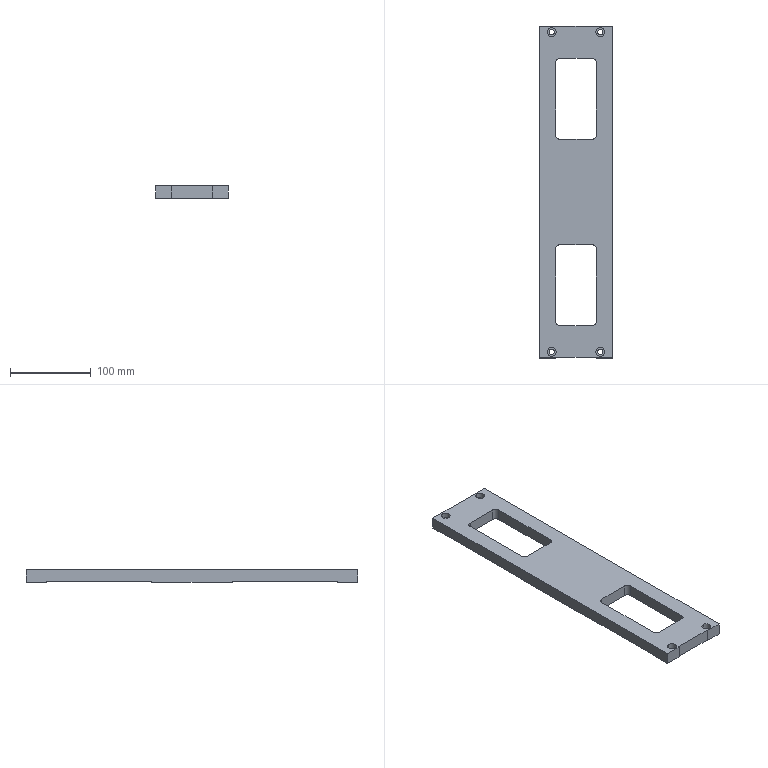NC program | NX | posted with a generic post | part box 90 x 410 x 15 mm
Whole program:
N10 G17 G21 G94 G90
(PLANAR_MILL_1_COPY_COPY , TOOL : D6A45)
N12 T07 M6
N14 G54
N16 G17 G0 G90 X-200.57 Y-28.539 S9500 M3
N18 G43 Z30. H7
N20 Z0.5
N22 G94 G1 Z-1. F1250.
N24 X-201.6 Y-29.134
N26 G3 X-202.1 Y-30. R1.
N28 X-197.5 Y-34.6 R4.6
N30 X-202.1 Y-30. R-4.6
N32 X-201.6 Y-30.866 R1.
N34 G1 X-200.57 Y-31.461
N36 Z0.5
N38 G0 Z30.
N40 Y31.461
N42 Z0.5
N44 G1 Z-1.
N46 X-201.6 Y30.866
N48 G3 X-202.1 Y30. R1.
N50 X-197.5 Y25.4 R4.6
N52 X-202.1 Y30. R-4.6
N54 X-201.6 Y29.134 R1.
N56 G1 X-200.57 Y28.539
N58 Z0.5
N60 G0 Z30.
N62 X-113.73 Y22.9
N64 Z0.5
N66 G1 Z-1.
N68 X-114.134 Y23.6
N70 G3 X-115. Y24.1 R1.
N72 G1 X-160.
N74 G3 X-164.1 Y20. R4.1
N76 G1 Y-20.
N78 G3 X-160. Y-24.1 R4.1
N80 G1 X-70.
N82 G3 X-65.9 Y-20. R4.1
N84 G1 Y20.
N86 G3 X-70. Y24.1 R4.1
N88 G1 X-115.
N90 G3 X-115.866 Y23.6 R1.
N92 G1 X-116.27 Y22.9
N94 Z0.5
N96 G0 Z30.
N98 X-1.27 Y47.1
N100 Z0.5
N102 G1 Z-1.
N104 X-0.866 Y46.4
N106 G3 X0. Y45.9 R1.
N108 G1 X204.9
N110 G2 X205.9 Y44.9 R1.
N112 G1 Y25.1
N114 G2 X204.9 Y24.1 R1.
N116 G1 Y-24.1
N118 G2 X205.9 Y-25.1 R1.
N120 G1 Y-44.9
N122 G2 X204.9 Y-45.9 R1.
N124 G1 X-204.9
N126 G2 X-205.9 Y-44.9 R1.
N128 G1 Y44.9
N130 G2 X-204.9 Y45.9 R1.
N132 G1 X0.
N134 G3 X0.866 Y46.4 R1.
N136 G1 X1.27 Y47.1
N138 Z0.5
N140 G0 Z30.
N142 X116.27 Y22.9
N144 Z0.5
N146 G1 Z-1.
N148 X115.866 Y23.6
N150 G3 X115. Y24.1 R1.
N152 G1 X70.
N154 G3 X65.9 Y20. R4.1
N156 G1 Y-20.
N158 G3 X70. Y-24.1 R4.1
N160 G1 X160.
N162 G3 X164.1 Y-20. R4.1
N164 G1 Y20.
N166 G3 X160. Y24.1 R4.1
N168 G1 X115.
N170 G3 X114.134 Y23.6 R1.
N172 G1 X113.73 Y22.9
N174 Z0.5
N176 G0 Z30.
N178 X200.57 Y28.539
N180 Z0.5
N182 G1 Z-1.
N184 X201.6 Y29.134
N186 G3 X202.1 Y30. R1.
N188 X197.5 Y34.6 R4.6
N190 X202.1 Y30. R-4.6
N192 X201.6 Y30.866 R1.
N194 G1 X200.57 Y31.461
N196 Z0.5
N198 G0 Z30.
N200 Y-31.461
N202 Z0.5
N204 G1 Z-1.
N206 X201.6 Y-30.866
N208 G3 X202.1 Y-30. R1.
N210 X197.5 Y-25.4 R4.6
N212 X202.1 Y-30. R-4.6
N214 X201.6 Y-29.134 R1.
N216 G1 X200.57 Y-28.539
N218 Z0.5
N220 G0 Z30.
N222 M5
N224 M2